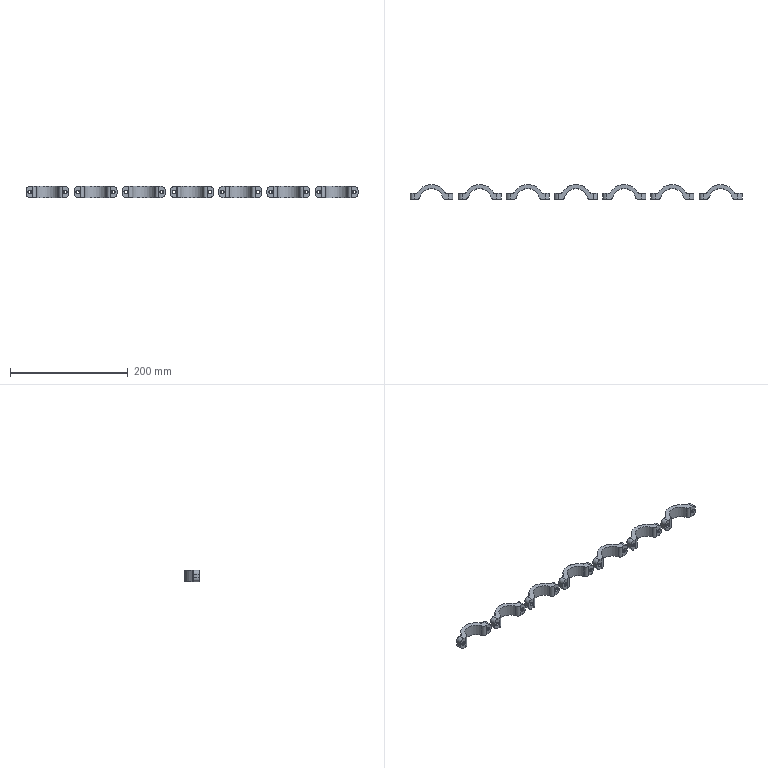NC program | Mastercam | posted with a generic post
Lines 2923 to 4896 of 23883, first 1623 of 1974 lines:
(16 CO |TOOL - 1|DIA. OFF. - 1|LEN. - 1|TOOL DIA. - 16.)
N5908 T1 M6
N5910 G0 G56 G90 X-44.884 Y-23.028 C0. B180. S6000 M3
N5912 G43 H1 Z40.
N5914 Z23.
N5916 G1 Z20.35 F2000.
N5918 X-45.357 Y-21.853 Z20.234 F4000.
N5920 G3 X-46.151 Y-20.651 Z20.1 I-3.34 J-1.343
N5922 G1 X-46.65 Y-19.858
N5924 G2 X-48.163 Y-14.465 I12.434 J6.398
N5926 X-48.3 Y-10.792 I49.344 J3.673
N5928 X-48.298 Y-10.346 I49.481
N5930 X-48.271 Y-4.938 I865.739 J-1.617
N5932 G1 X-48.266 Y-4.342
N5934 X-48.146 Y12.852
N5936 G2 X-47.9 Y14.539 I7.703 J-.262
N5938 X-46.414 Y17.572 I8.353 J-2.211
N5940 X-43.642 Y20.06 I7.961 J-6.083
N5942 X-39.47 Y21.708 I7.094 J-11.854
N5944 X-35.506 Y22.258 I5.523 J-25.257
N5946 X-30.242 Y22.416 I5.264 J-87.34
N5948 X-29.657 Y22.414 J-87.498
N5950 X-22.977 Y22.386 I-.5 J-912.012
N5952 G1 X-22.373 Y22.382
N5954 X33.907 Y22.008
N5956 X34.201 Y22.009
N5958 G2 X37.187 Y21.983 J-172.847
N5960 X40.482 Y20.969 I-.705 J-8.148
N5962 X43.577 Y18.308 I-5.14 J-9.11
N5964 X45.609 Y14.702 I-11.006 J-8.578
N5966 X46.723 Y10.602 I-19.798 J-7.578
N5968 X47.299 Y4.944 I-46.088 J-7.548
N5970 X47.479 Y-3.923 I-217.933 J-8.867
N5972 G1 Y-3.929
N5974 G2 X47.489 Y-6.4 I-975.272 J-5.162
N5976 G1 X47.49 Y-7.016
N5978 G2 X47.494 Y-9.105 I-595.573 J-2.089
N5980 X47.49 Y-11.453 I-595.577
N5982 X46.583 Y-14.751 I-8.028 J.432
N5984 X43.991 Y-17.922 I-9.082 J4.78
N5986 X39.944 Y-20.204 I-8.744 J10.774
N5988 X35.874 Y-21.26 I-7.5 J20.538
N5990 X30.245 Y-21.807 I-7.504 J47.966
N5992 X21.392 Y-21.979 I-8.853 J227.798
N5994 G1 X21.385
N5996 G2 X19.531 Y-21.987 I-4.737 J921.856
N5998 G1 X18.915 Y-21.989
N6000 X-36.463 Y-21.993
N6002 G2 X-40.392 Y-20.823 I.404 J8.545
N6004 X-43.439 Y-18.134 I5.427 J9.217
N6006 X-45.439 Y-14.523 I11.134 J8.529
N6008 X-46.528 Y-10.416 I19.842 J7.456
N6010 X-47.067 Y-4.751 I45.995 J7.238
N6012 X-47.192 Y2.627 I217.088 J7.378
N6014 X-47.187 Y4.123 I217.213
N6016 X-47.18 Y6.594 I970.906 J-1.502
N6018 G1 X-47.178 Y7.21
N6020 G2 X-47.155 Y9.304 I114.207 J-.216
N6022 X-44.591 Y15.696 I10.476 J-.491
N6024 X-40.819 Y18.674 I9.729 J-8.446
N6026 X-36.989 Y20.159 I8.291 J-15.701
N6028 X-32.412 Y20.97 I7.487 J-28.95
N6030 X-26.367 Y21.299 I6.984 J-72.475
N6032 X-19.406 Y21.346 I6.961 J-512.395
N6034 X-14.54 Y21.324 J-512.442
N6036 G1 X-13.926 Y21.32
N6038 X33.206 Y21.005
N6040 G2 X40.416 Y18.047 I-.442 J-11.343
N6042 X43.518 Y13.986 I-9.563 J-10.518
N6044 X45.177 Y9.517 I-18.069 J-9.253
N6046 X46.028 Y4.379 I-34.271 J-8.311
N6048 X46.404 Y-2.851 I-94.948 J-8.563
N6050 X46.464 Y-7.318 I-291.246 J-6.155
N6052 X43.757 Y-14.636 I-11.254 J.003
N6054 X39.738 Y-17.867 I-10.573 J9.037
N6056 X35.25 Y-19.611 I-9.342 J17.402
N6058 X30.082 Y-20.504 I-8.375 J33.036
N6060 X23.468 Y-20.883 I-8.361 J88.08
N6062 X12.151 Y-20.995 I-11.317 J576.455
N6064 X11.038 Y-20.993 J576.566
N6066 G1 X10.423 Y-20.994
N6068 X-32.667 Y-20.995
N6070 G2 X-40.331 Y-17.889 I.182 J11.455
N6072 X-43.371 Y-13.804 I9.797 J10.466
N6074 X-44.985 Y-9.33 I18.285 J9.126
N6076 X-45.795 Y-4.192 I34.546 J8.076
N6078 X-46.12 Y3.038 I95.438 J7.911
N6080 X-46.139 Y5.321 I135.435 J2.283
N6082 G1 Y5.679
N6084 G2 X-45.662 Y9.236 I13.643 J-.018
N6086 X-42.309 Y14.816 I11.969 J-3.393
N6088 X-38.661 Y17.41 I10.477 J-10.873
N6090 X-33.842 Y19.148 I9.553 J-18.94
N6092 X-28.045 Y20.004 I8.556 J-37.876
N6094 X-20.243 Y20.292 I8.196 J-116.201
N6096 X-14.949 Y20.306 I5.294 J-980.054
N6098 X-6.64 Y20.272 J-980.068
N6100 G1 X-6.026 Y20.267
N6102 X29.631 Y20.027
N6104 G2 X32.943 Y19.666 I-.08 J-16.055
N6106 X39.744 Y15.722 I-2.916 J-12.866
N6108 X42.235 Y12.172 I-11.816 J-10.939
N6110 X44.013 Y7.445 I-19.674 J-10.101
N6112 X44.986 Y1.662 I-37.574 J-9.294
N6114 X45.331 Y-4.52 I-76.625 J-7.38
N6116 G1 Y-4.572
N6118 G2 X44.35 Y-9.632 I-13.534
N6120 X40.614 Y-14.709 I-12.401 J5.213
N6122 X36.622 Y-17.211 I-10.844 J12.861
N6124 X31.942 Y-18.74 I-9.756 J21.949
N6126 X26.25 Y-19.565 I-9.037 J42.276
N6128 X18.472 Y-19.911 I-9.295 J121.207
N6130 X5.449 Y-19.998 I-13.023 J981.766
N6132 X3.633 Y-19.996 J981.852
N6134 G1 X3.019 Y-19.997
N6136 X-29.668 Y-19.988
N6138 G2 X-33.578 Y-19.409 I.23 J15.043
N6140 X-39.75 Y-15.436 I3.847 J12.756
N6142 X-42.342 Y-11.461 I12.349 J10.885
N6144 X-43.932 Y-6.754 I21.156 J9.768
N6146 X-44.776 Y-1.022 I40.362 J8.873
N6148 X-44.986 Y3.21 I56.386 J4.914
N6150 G1 Y3.27
N6152 G2 X-44.508 Y7.095 I15.548
N6154 X-40.431 Y13.721 I13.097 J-3.49
N6156 X-36.503 Y16.346 I11.107 J-12.37
N6158 X-31.807 Y17.997 I9.983 J-20.892
N6160 X-26.055 Y18.897 I9.071 J-39.163
N6162 X-18.221 Y19.248 I8.743 J-107.429
N6164 X-10.9 Y19.282 I7.321 J-771.653
N6166 X-3.975 Y19.252 J-771.688
N6168 G1 X-3.361 Y19.247
N6170 X26.781 Y19.041
N6172 G2 X30.135 Y18.763 I-.157 J-22.182
N6174 X38.782 Y13.854 I-2.371 J-14.247
N6176 X41.647 Y9.224 I-13.729 J-11.7
N6178 X43.283 Y3.902 I-24.295 J-10.377
N6180 X43.984 Y-1.194 I-40.547 J-8.179
N6182 X44.032 Y-2.454 I-16.613 J-1.26
N6184 X43.845 Y-4.947 I-16.661
N6186 X39.813 Y-12.677 I-13.559 J2.155
N6188 X35.994 Y-15.454 I-11.605 J11.941
N6190 X31.333 Y-17.29 I-10.585 J20.049
N6192 X25.548 Y-18.365 I-9.808 J36.689
N6194 X18.292 Y-18.838 I-9.436 J88.748
N6196 X6.377 Y-18.988 I-11.915 J476.068
N6198 G1 X5.836 Y-18.987
N6200 X5.221 Y-18.989
N6202 X-26.132 Y-18.996
N6204 X-26.274 Y-18.997
N6206 G2 X-29.815 Y-18.736 J24.22
N6208 X-38.503 Y-13.872 I2.246 J14.205
N6210 X-41.025 Y-10.018 I13.181 J11.376
N6212 X-42.862 Y-4.63 I22.04 J10.522
N6214 X-43.62 Y.675 I32.605 J7.367
N6216 X-43.646 Y1.583 I16.129 J.908
N6218 X-43.281 Y4.996 I16.155
N6220 X-39.255 Y12.078 I13.734 J-3.122
N6222 X-35.448 Y14.821 I11.701 J-12.225
N6224 X-30.793 Y16.651 I10.619 J-20.178
N6226 X-24.996 Y17.724 I9.721 J-36.329
N6228 X-17.721 Y18.175 I8.973 J-85.833
N6230 X-9.051 Y18.265 I8.67 J-416.715
N6232 X-5.867 Y18.253 J-416.805
N6234 G1 X-5.251 Y18.25
N6236 X24.308 Y18.053
N6238 G2 X28.281 Y17.719 I-.281 J-27.075
N6240 X37.8 Y12.131 I-2.537 J-15.223
N6242 X40.684 Y7.207 I-15.183 J-12.199
N6244 X42.373 Y.943 I-24.077 J-9.853
N6246 X42.521 Y-1.199 I-15.427 J-2.142
N6248 X42.36 Y-3.43 I-15.575
N6250 X38.48 Y-11.166 I-13.844 J2.102
N6252 X34.754 Y-14.034 I-12.038 J11.786
N6254 X30.132 Y-16.005 I-11.068 J19.551
N6256 X24.322 Y-17.219 I-10.291 J34.76
N6258 X17.011 Y-17.787 I-9.856 J79.506
N6260 X5.747 Y-17.975 I-11.505 J350.541
N6262 G1 X5.13 Y-17.979
N6264 X-23.151 Y-17.997
N6266 X-23.307 Y-17.998
N6268 G2 X-26.853 Y-17.834 J38.682
N6270 X-31.433 Y-16.701 I1.631 J16.421
N6272 X-37.658 Y-11.971 I5.985 J14.336
N6274 X-40.331 Y-7.413 I15.207 J11.981
N6276 X-41.916 Y-1.779 I21.451 J9.077
N6278 X-42.085 Y.483 I15.043 J2.262
N6280 X-41.854 Y3.127 I15.212
N6282 X-38.138 Y10.37 I13.894 J-2.553
N6284 X-34.443 Y13.281 I12.146 J-11.614
N6286 X-29.818 Y15.303 I11.138 J-19.183
N6288 X-23.981 Y16.547 I10.247 J-33.756
N6290 X-16.638 Y17.109 I9.482 J-75.712
N6292 X-7.264 Y17.244 I9.374 J-324.031
N6294 X-5.355 Y17.238 J-324.167
N6296 G1 X-4.737 Y17.237
N6298 X20.461 Y17.087
N6300 X20.546 Y17.088
N6302 G2 X24.644 Y16.932 J-54.062
N6304 X28.969 Y16.079 I-1.525 J-19.123
N6306 X36.14 Y11.319 I-5.025 J-15.352
N6308 X39.713 Y5.273 I-14.857 J-12.86
N6310 X40.707 Y1.143 I-15.557 J-5.927
N6312 X40.786 Y-.32 I-13.573 J-1.463
N6314 X37.607 Y-9.076 I-13.652
N6316 X34.032 Y-12.278 I-12.441 J10.295
N6318 X29.438 Y-14.551 I-11.6 J17.67
N6320 X23.563 Y-16.004 I-10.813 J31.123
N6322 X16.813 Y-16.679 I-10.074 J66.612
N6324 X6.702 Y-16.949 I-11.173 J228.959
N6326 X-.09 Y-16.986 I-8.808 J997.7
N6328 G1 X-.706 Y-16.988
N6330 X-21.016 Y-16.994
N6332 G2 X-24.622 Y-16.844 I.04 J44.664
N6334 X-29.005 Y-15.932 I1.558 J18.48
N6336 X-35.794 Y-11.389 I5.229 J15.156
N6338 X-39.84 Y-3.807 I13.83 J12.252
N6340 X-40.286 Y-.322 I13.407 J3.485
N6342 X-39.777 Y3.396 I13.853
N6344 X-36.113 Y9.533 I13.638 J-3.981
N6346 X-32.018 Y12.544 I12.215 J-12.321
N6348 X-26.682 Y14.601 I11.262 J-21.27
N6350 X-20.282 Y15.705 I10.275 J-40.457
N6352 X-12.433 Y16.143 I9.662 J-102.647
N6354 X-3.307 Y16.225 I9.126 J-507.263
N6356 X.629 Y16.21 J-507.345
N6358 G1 X1.245 Y16.207
N6360 X19.105 Y16.09
N6362 G2 X23.376 Y15.87 I-.217 J-45.652
N6364 X28.067 Y14.801 I-1.99 J-19.558
N6366 X36.683 Y7.65 I-5.93 J-15.91
N6368 X38.641 Y2.437 I-12.424 J-7.643
N6370 X38.804 Y.393 I-12.752 J-2.044
N6372 X36.615 Y-6.801 I-12.915
N6374 X32.866 Y-10.713 I-13.001 J8.707
N6376 X28.293 Y-13.215 I-11.853 J16.237
N6378 X23.092 Y-14.706 I-10.725 J27.591
N6380 X16.232 Y-15.569 I-10.502 J55.778
N6382 X7.293 Y-15.909 I-10.803 J166.404
N6384 X-5.24 Y-15.992 I-12.533 J949.534
N6386 X-5.685 Y-15.991 J949.617
N6388 G1 X-6.3 Y-15.993
N6390 X-19.273 Y-15.986
N6392 G2 X-23.662 Y-15.731 I.05 J38.732
N6394 X-28.427 Y-14.504 I2.225 J18.517
N6396 X-36.816 Y-6.792 I6.235 J15.199
N6398 X-38.235 Y-.894 I11.551 J5.898
N6400 X-38.205 Y-.032 I12.97
N6402 X-35.873 Y6.469 I12.933 J-.971
N6404 X-31.683 Y10.536 I12.669 J-8.861
N6406 X-27.085 Y12.828 I11.61 J-17.534
N6408 X-21.203 Y14.292 I10.813 J-30.899
N6410 X-14.437 Y14.965 I9.881 J-64.995
N6412 X-4.472 Y15.197 I9.965 J-213.659
N6414 G1 X-4.304
N6416 G2 X-1.177 Y15.202 I3.127 J-959.648
N6418 X3.726 Y15.189 J-959.653
N6420 G1 X4.342 Y15.186
N6422 X17.31 Y15.096
N6424 G2 X21.539 Y14.876 I-.44 J-48.99
N6426 X26.532 Y13.772 I-2.04 J-21.08
N6428 X32.909 Y9.668 I-5.584 J-15.683
N6430 X35.954 Y4.72 I-9.601 J-9.319
N6432 X36.567 Y.947 I-11.302 J-3.773
N6434 X35.493 Y-3.998 I-11.915
N6436 X31.799 Y-8.9 I-13.003 J5.955
N6438 X27.621 Y-11.598 I-11.773 J13.646
N6440 X22.343 Y-13.406 I-11.099 J23.794
N6442 X16.048 Y-14.398 I-10.441 J45.811
N6444 X7.631 Y-14.852 I-10.685 J119.676
N6446 X-6.332 Y-14.99 I-13.963 J708.147
N6448 X-7.245 Y-14.989 J708.285
N6450 G1 X-7.859 Y-14.991
N6452 G2 X-11.297 Y-14.997 I-3.438 J898.451
N6454 X-17.808 Y-14.973 J898.458
N6456 X-22.206 Y-14.679 I.336 J38.047
N6458 X-27.313 Y-13.295 I2.468 J19.22
N6460 X-32.535 Y-9.681 I6.197 J14.535
N6462 X-35.506 Y-4.471 I8.96 J8.561
N6464 X-35.909 Y-1.431 I11.273 J3.04
N6466 X-34.928 Y3.252 I11.676
N6468 X-31.62 Y7.897 I12.723 J-5.563
N6470 X-27.836 Y10.559 I11.701 J-12.605
N6472 X-22.503 Y12.57 I11.191 J-21.605
N6474 X-16.129 Y13.653 I10.357 J-41.682
N6476 X-8.292 Y14.097 I9.87 J-104.79
N6478 X1.247 Y14.19 I9.539 J-487.809
N6480 X4.776 Y14.177 J-487.902
N6482 G1 X5.392 Y14.175
N6484 X15.295 Y14.107
N6486 G2 X20.201 Y13.836 I-.461 J-52.82
N6488 X25.141 Y12.714 I-2.345 J-21.763
N6490 X29.399 Y10.429 I-5.404 J-15.179
N6492 X32.681 Y6.689 I-7.346 J-9.755
N6494 X34.027 Y1.433 I-9.587 J-5.256
N6496 X33.71 Y-1.177 I-10.933
N6498 X30.967 Y-6.439 I-12.307 J3.07
N6500 X27.264 Y-9.575 I-11.897 J10.295
N6502 X22.644 Y-11.699 I-11.3 J18.495
N6504 X16.823 Y-13.033 I-10.744 J33.49
N6506 X9.478 Y-13.702 I-10.466 J74.315
N6508 X-1.211 Y-13.952 I-11.702 J271.761
N6510 X-5.534 Y-13.977 I-7.889 J968.44
N6512 G1 X-6.15 Y-13.98
N6514 G2 X-10.115 Y-13.993 I-3.965 J647.904
N6516 X-16.127 Y-13.964 J647.916
N6518 X-20.481 Y-13.674 I.508 J40.507
N6520 X-25.085 Y-12.561 I2.503 J20.423
N6522 X-29.05 Y-10.367 I5.164 J14.011
N6524 X-32.502 Y-5.828 I6.779 J8.738
N6526 X-33.253 Y-1.88 I10.007 J3.948
N6528 X-32.848 Y1.044 I10.758
N6530 X-29.926 Y6.207 I12.193 J-3.491
N6532 X-26.541 Y8.972 I11.59 J-10.732
N6534 X-21.897 Y11.078 I11.131 J-18.371
N6536 X-16.063 Y12.374 I10.49 J-33.447
N6538 X-8.714 Y12.991 I9.952 J-74.522
N6540 X1.47 Y13.17 I10.184 J-289.084
N6542 X2.595 Y13.168 J-289.263
N6544 G1 X3.181
N6546 G2 X5.683 Y13.165 J-974.104
N6548 G1 X6.299 Y13.163
N6550 G2 X14.421 Y13.093 I-.2 J-495.657
N6552 X19.441 Y12.724 I-.758 J-44.556
N6554 X24.05 Y11.546 I-2.741 J-20.34
N6556 X27.769 Y9.321 I-4.444 J-11.647
N6558 X31.128 Y1.893 I-6.534 J-7.428
N6560 X31.065 Y.782 I-9.893
N6562 X29.087 Y-4.48 I-11.427 J1.293
N6564 X25.098 Y-8.36 I-11.91 J8.252
N6566 X20.429 Y-10.631 I-11.181 J17.052
N6568 X14.562 Y-12.02 I-10.652 J31.926
N6570 X7.201 Y-12.699 I-10.409 J72.593
N6572 X-3.49 Y-12.95 I-11.721 J270.501
N6574 X-8.431 Y-12.979 I-8.146 J995.561
N6576 X-10.273 Y-12.987 I-1.842 J217.156
N6578 X-15.437 Y-12.925 J217.164
N6580 X-19.911 Y-12.508 I.967 J34.557
N6582 X-23.388 Y-11.595 I3.045 J18.675
N6584 X-26.785 Y-9.655 I4.018 J10.981
N6586 X-30.2 Y-2.348 I6.11 J7.307
N6588 X-30.179 Y-1.707 I9.525
N6590 X-28.651 Y3.21 I10.99 J-.718
N6592 X-25.167 Y7.101 I11.871 J-7.125
N6594 X-20.83 Y9.54 I10.916 J-14.334
N6596 X-15.553 Y11.043 I10.265 J-26.021
N6598 X-9.344 Y11.807 I9.647 J-52.804
N6600 X-.376 Y12.122 I9.935 J-154.892
N6602 X5.109 Y12.151 I5.485 J-507.313
N6604 X12.749 Y12.094 J-507.343
N6606 X17.724 Y11.744 I-.845 J-47.461
N6608 X21.171 Y10.989 I-2.554 J-19.925
N6610 X24.261 Y9.402 I-3.121 J-9.877
N6612 X27.69 Y3.33 I-5.382 J-7.043
N6614 X27.751 Y2.225 I-10.015 J-1.105
N6616 X26.881 Y-1.871 I-10.076
N6618 X23.658 Y-6.234 I-11.547 J5.157
N6620 X20.482 Y-8.416 I-10.607 J12.04
N6622 X15.806 Y-10.22 I-10.458 J20.141
N6624 X10.066 Y-11.276 I-10.048 J38.489
N6626 X2.194 Y-11.802 I-10.464 J97.405
N6628 X-8.792 Y-11.961 I-10.986 J380.97
N6630 X-12.892 Y-11.938 J381.128
N6632 X-17.181 Y-11.663 I.699 J44.352
N6634 X-20.313 Y-11.033 I2.009 J18.109
N6636 X-23.444 Y-9.401 I2.658 J8.919
N6638 X-26.524 Y-3.846 I5.38 J6.613
N6640 X-26.601 Y-2.626 I9.663 J1.22
N6642 X-25.964 Y.839 I9.74
N6644 X-23.234 Y5.036 I11.108 J-4.237
N6646 X-19.251 Y7.897 I10.824 J-10.866
N6648 X-14.551 Y9.63 I10.162 J-20.324
N6650 X-8.814 Y10.606 I9.626 J-39.224
N6652 X-.957 Y11.051 I9.674 J-101.283
N6654 X5.912 Y11.129 I6.869 J-300.508
N6656 X11.667 Y11.074 J-300.586
N6658 X15.977 Y10.764 I-1.019 J-44.25
N6660 X17.981 Y10.363 I-1.681 J-13.615
N6662 X23.406 Y4.909 I-2.127 J-7.542
N6664 X23.734 Y2.494 I-8.716 J-2.415
N6666 X23.437 Y.193 I-9.044
N6668 X21.003 Y-4.332 I-10.676 J2.826
N6670 X17.017 Y-7.468 I-10.778 J9.596
N6672 X12.263 Y-9.323 I-10.131 J18.951
N6674 X6.496 Y-10.347 I-9.69 J37.822
N6676 X-1.357 Y-10.828 I-10.18 J101.794
N6678 X-8.344 Y-10.934 I-6.987 J230.985
N6680 X-11.519 Y-10.912 J231.091
N6682 X-15.621 Y-10.633 I.545 J38.365
N6684 X-18.767 Y-9.503 I.995 J7.712
N6686 X-21.752 Y-5.687 I4.02 J6.221
N6688 X-22.216 Y-2.894 I8.179 J2.793
N6690 X-22.121 Y-1.613 I8.643
N6692 X-20.37 Y2.726 I10.081 J-1.544
N6694 X-16.915 Y6.073 I10.543 J-7.43
N6696 X-12.808 Y8.088 I9.767 J-14.71
N6698 X-7.517 Y9.344 I9.316 J-27.474
N6700 X-.743 Y9.94 I9.195 J-65.666
N6702 X6.41 Y10.089 I7.153 J-171.222
N6704 X10.826 Y10.033 J-171.371
N6706 X12.753 Y9.913 I-1.151 J-34.045
N6708 X13.754 Y9.713 I-.842 J-6.828
N6710 G1 X14.603 Y9.411
N6712 X15.39 Y9.
N6714 X16.119 Y8.477
N6716 G2 X18.322 Y5.039 I-4.431 J-5.264
N6718 X18.625 Y2.776 I-8.29 J-2.263
N6720 X18.438 Y.991 I-8.593
N6722 X16.434 Y-3.24 I-10.097 J2.192
N6724 X12.821 Y-6.372 I-10.176 J8.088
N6726 X9.101 Y-8.046 I-9.239 J15.564
N6728 X3.832 Y-9.213 I-9.092 J28.559
N6730 X-2.891 Y-9.763 I-9.224 J71.369
N6732 X-8.012 Y-9.878 I-5.121 J114.655
N6734 X-10.77 Y-9.845 J114.769
N6736 G1 X-11.566 Y-9.738
N6738 X-12.295 Y-9.537
N6740 X-12.985 Y-9.243
N6742 X-13.644 Y-8.848
N6744 X-14.269 Y-8.344
N6746 X-14.843 Y-7.722
N6748 X-15.35 Y-6.986
N6750 G2 X-16.272 Y-3.969 I6.141 J3.526
N6752 X-16.295 Y-3.333 I8.713 J.636
N6754 X-15.821 Y-.496 I8.736
N6756 X-13.004 Y3.895 I10.488 J-3.63
N6758 X-9.179 Y6.493 I9.679 J-10.136
N6760 X-5.114 Y7.887 I8.659 J-18.622
N6762 X-.007 Y8.687 I8.217 J-35.776
N6764 X6.605 Y8.997 I7.077 J-80.228
N6766 X9.31 Y8.169 I-.233 J-5.595
N6768 G1 X9.945 Y7.713
N6770 X10.589 Y7.085
N6772 G2 X11.721 Y5.132 I-4.66 J-4.002
N6774 X12.174 Y2.494 I-7.455 J-2.638
N6776 X12.145 Y1.817 I-7.908
N6778 X11.127 Y-1.627 I-8.967 J.776
N6780 X8.175 Y-5.172 I-9.983 J5.312
N6782 X4.425 Y-7.28 I-8.554 J10.827
N6784 X.345 Y-8.366 I-7.583 J20.295
N6786 X-3.662 Y-8.825 I-6.319 J37.465
N6788 X-3.794 Y-8.827 I-.132 J5.599
N6790 X-5.835 Y-8.441 J5.601
N6792 G1 X-6.596 Y-8.075
N6794 G2 X-8.035 Y-6.883 I2.904 J4.972
N6796 X-8.879 Y-5.612 I4.798 J4.098
N6798 G1 X-9.211 Y-4.847
N6800 X-9.468 Y-3.997
N6802 X-9.631 Y-3.083
N6804 X-9.686 Y-2.119
N6806 X-9.625 Y-1.132
N6808 X-9.449 Y-.146
N6810 X-9.161 Y.813
N6812 X-8.776 Y1.724
N6814 G2 X-7.2 Y4.036 I8.815 J-4.317
N6816 X-3.546 Y6.713 I8.652 J-7.976
N6818 X-1.693 Y7.421 I4.944 J-10.154
N6820 G1 X1.801 Y8.289 Z20.35
N6822 G0 Z40.
N6824 X-44.884 Y-23.028
N6826 Z23.
N6828 G1 Z20.35 F2000.
N6830 X-45.357 Y-21.853 Z20.234 F4000.
N6832 G3 X-46.151 Y-20.651 Z20.1 I-3.34 J-1.343
N6834 G1 X-46.65 Y-19.858
N6836 G2 X-48.163 Y-14.465 I12.434 J6.398
N6838 X-48.3 Y-10.792 I49.344 J3.673
N6840 X-48.298 Y-10.346 I49.481
N6842 X-48.271 Y-4.938 I865.739 J-1.617
N6844 G1 X-48.266 Y-4.342
N6846 X-48.146 Y12.852
N6848 G2 X-47.9 Y14.539 I7.703 J-.262
N6850 X-46.414 Y17.572 I8.353 J-2.211
N6852 X-43.642 Y20.06 I7.961 J-6.083
N6854 X-39.47 Y21.708 I7.094 J-11.854
N6856 X-35.506 Y22.258 I5.523 J-25.257
N6858 X-30.242 Y22.416 I5.264 J-87.34
N6860 X-29.657 Y22.414 J-87.498
N6862 X-22.977 Y22.386 I-.5 J-912.012
N6864 G1 X-22.373 Y22.382
N6866 X33.907 Y22.008
N6868 X34.201 Y22.009
N6870 G2 X37.187 Y21.983 J-172.847
N6872 X40.482 Y20.969 I-.705 J-8.148
N6874 X43.577 Y18.308 I-5.14 J-9.11
N6876 X45.609 Y14.702 I-11.006 J-8.578
N6878 X46.723 Y10.602 I-19.798 J-7.578
N6880 X47.299 Y4.944 I-46.088 J-7.548
N6882 X47.479 Y-3.923 I-217.933 J-8.867
N6884 G1 Y-3.929
N6886 G2 X47.489 Y-6.4 I-975.272 J-5.162
N6888 G1 X47.49 Y-7.016
N6890 G2 X47.494 Y-9.105 I-595.573 J-2.089
N6892 X47.49 Y-11.453 I-595.577
N6894 X46.583 Y-14.751 I-8.028 J.432
N6896 X43.991 Y-17.922 I-9.082 J4.78
N6898 X39.944 Y-20.204 I-8.744 J10.774
N6900 X35.874 Y-21.26 I-7.5 J20.538
N6902 X30.245 Y-21.807 I-7.504 J47.966
N6904 X21.392 Y-21.979 I-8.853 J227.798
N6906 G1 X21.385
N6908 G2 X19.531 Y-21.987 I-4.737 J921.856
N6910 G1 X18.915 Y-21.989
N6912 X-36.463 Y-21.993
N6914 G2 X-40.392 Y-20.823 I.404 J8.545
N6916 X-43.439 Y-18.134 I5.427 J9.217
N6918 X-45.439 Y-14.523 I11.134 J8.529
N6920 X-46.528 Y-10.416 I19.842 J7.456
N6922 X-47.067 Y-4.751 I45.995 J7.238
N6924 X-47.192 Y2.627 I217.088 J7.378
N6926 X-47.187 Y4.123 I217.213
N6928 X-47.18 Y6.594 I970.906 J-1.502
N6930 G1 X-47.178 Y7.21
N6932 G2 X-47.155 Y9.304 I114.207 J-.216
N6934 X-44.591 Y15.696 I10.476 J-.491
N6936 X-40.819 Y18.674 I9.729 J-8.446
N6938 X-36.989 Y20.159 I8.291 J-15.701
N6940 X-32.412 Y20.97 I7.487 J-28.95
N6942 X-26.367 Y21.299 I6.984 J-72.475
N6944 X-19.406 Y21.346 I6.961 J-512.395
N6946 X-14.54 Y21.324 J-512.442
N6948 G1 X-13.926 Y21.32
N6950 X33.206 Y21.005
N6952 G2 X40.416 Y18.047 I-.442 J-11.343
N6954 X43.518 Y13.986 I-9.563 J-10.518
N6956 X45.177 Y9.517 I-18.069 J-9.253
N6958 X46.028 Y4.379 I-34.271 J-8.311
N6960 X46.404 Y-2.851 I-94.948 J-8.563
N6962 X46.464 Y-7.318 I-291.246 J-6.155
N6964 X43.757 Y-14.636 I-11.254 J.003
N6966 X39.738 Y-17.867 I-10.573 J9.037
N6968 X35.25 Y-19.611 I-9.342 J17.402
N6970 X30.082 Y-20.504 I-8.375 J33.036
N6972 X23.468 Y-20.883 I-8.361 J88.08
N6974 X12.151 Y-20.995 I-11.317 J576.455
N6976 X11.038 Y-20.993 J576.566
N6978 G1 X10.423 Y-20.994
N6980 X-32.667 Y-20.995
N6982 G2 X-40.331 Y-17.889 I.182 J11.455
N6984 X-43.371 Y-13.804 I9.797 J10.466
N6986 X-44.985 Y-9.33 I18.285 J9.126
N6988 X-45.795 Y-4.192 I34.546 J8.076
N6990 X-46.12 Y3.038 I95.438 J7.911
N6992 X-46.139 Y5.321 I135.435 J2.283
N6994 G1 Y5.679
N6996 G2 X-45.662 Y9.236 I13.643 J-.018
N6998 X-42.309 Y14.816 I11.969 J-3.393
N7000 X-38.661 Y17.41 I10.477 J-10.873
N7002 X-33.842 Y19.148 I9.553 J-18.94
N7004 X-28.045 Y20.004 I8.556 J-37.876
N7006 X-20.243 Y20.292 I8.196 J-116.201
N7008 X-14.949 Y20.306 I5.294 J-980.054
N7010 X-6.64 Y20.272 J-980.068
N7012 G1 X-6.026 Y20.267
N7014 X29.631 Y20.027
N7016 G2 X32.943 Y19.666 I-.08 J-16.055
N7018 X39.744 Y15.722 I-2.916 J-12.866
N7020 X42.235 Y12.172 I-11.816 J-10.939
N7022 X44.013 Y7.445 I-19.674 J-10.101
N7024 X44.986 Y1.662 I-37.574 J-9.294
N7026 X45.331 Y-4.52 I-76.625 J-7.38
N7028 G1 Y-4.572
N7030 G2 X44.35 Y-9.632 I-13.534
N7032 X40.614 Y-14.709 I-12.401 J5.213
N7034 X36.622 Y-17.211 I-10.844 J12.861
N7036 X31.942 Y-18.74 I-9.756 J21.949
N7038 X26.25 Y-19.565 I-9.037 J42.276
N7040 X18.472 Y-19.911 I-9.295 J121.207
N7042 X5.449 Y-19.998 I-13.023 J981.766
N7044 X3.633 Y-19.996 J981.852
N7046 G1 X3.019 Y-19.997
N7048 X-29.668 Y-19.988
N7050 G2 X-33.578 Y-19.409 I.23 J15.043
N7052 X-39.75 Y-15.436 I3.847 J12.756
N7054 X-42.342 Y-11.461 I12.349 J10.885
N7056 X-43.932 Y-6.754 I21.156 J9.768
N7058 X-44.776 Y-1.022 I40.362 J8.873
N7060 X-44.986 Y3.21 I56.386 J4.914
N7062 G1 Y3.27
N7064 G2 X-44.508 Y7.095 I15.548
N7066 X-40.431 Y13.721 I13.097 J-3.49
N7068 X-36.503 Y16.346 I11.107 J-12.37
N7070 X-31.807 Y17.997 I9.983 J-20.892
N7072 X-26.055 Y18.897 I9.071 J-39.163
N7074 X-18.221 Y19.248 I8.743 J-107.429
N7076 X-10.9 Y19.282 I7.321 J-771.653
N7078 X-3.975 Y19.252 J-771.688
N7080 G1 X-3.361 Y19.247
N7082 X26.781 Y19.041
N7084 G2 X30.135 Y18.763 I-.157 J-22.182
N7086 X38.782 Y13.854 I-2.371 J-14.247
N7088 X41.647 Y9.224 I-13.729 J-11.7
N7090 X43.283 Y3.902 I-24.295 J-10.377
N7092 X43.984 Y-1.194 I-40.547 J-8.179
N7094 X44.032 Y-2.454 I-16.613 J-1.26
N7096 X43.845 Y-4.947 I-16.661
N7098 X39.813 Y-12.677 I-13.559 J2.155
N7100 X35.994 Y-15.454 I-11.605 J11.941
N7102 X31.333 Y-17.29 I-10.585 J20.049
N7104 X25.548 Y-18.365 I-9.808 J36.689
N7106 X18.292 Y-18.838 I-9.436 J88.748
N7108 X6.377 Y-18.988 I-11.915 J476.068
N7110 G1 X5.836 Y-18.987
N7112 X5.221 Y-18.989
N7114 X-26.132 Y-18.996
N7116 X-26.274 Y-18.997
N7118 G2 X-29.815 Y-18.736 J24.22
N7120 X-38.503 Y-13.872 I2.246 J14.205
N7122 X-41.025 Y-10.018 I13.181 J11.376
N7124 X-42.862 Y-4.63 I22.04 J10.522
N7126 X-43.62 Y.675 I32.605 J7.367
N7128 X-43.646 Y1.583 I16.129 J.908
N7130 X-43.281 Y4.996 I16.155
N7132 X-39.255 Y12.078 I13.734 J-3.122
N7134 X-35.448 Y14.821 I11.701 J-12.225
N7136 X-30.793 Y16.651 I10.619 J-20.178
N7138 X-24.996 Y17.724 I9.721 J-36.329
N7140 X-17.721 Y18.175 I8.973 J-85.833
N7142 X-9.051 Y18.265 I8.67 J-416.715
N7144 X-5.867 Y18.253 J-416.805
N7146 G1 X-5.251 Y18.25
N7148 X24.308 Y18.053
N7150 G2 X28.281 Y17.719 I-.281 J-27.075
N7152 X37.8 Y12.131 I-2.537 J-15.223
N7154 X40.684 Y7.207 I-15.183 J-12.199
N7156 X42.373 Y.943 I-24.077 J-9.853
N7158 X42.521 Y-1.199 I-15.427 J-2.142
N7160 X42.36 Y-3.43 I-15.575
N7162 X38.48 Y-11.166 I-13.844 J2.102
N7164 X34.754 Y-14.034 I-12.038 J11.786
N7166 X30.132 Y-16.005 I-11.068 J19.551
N7168 X24.322 Y-17.219 I-10.291 J34.76
N7170 X17.011 Y-17.787 I-9.856 J79.506
N7172 X5.747 Y-17.975 I-11.505 J350.541
N7174 G1 X5.13 Y-17.979
N7176 X-23.151 Y-17.997
N7178 X-23.307 Y-17.998
N7180 G2 X-26.853 Y-17.834 J38.682
N7182 X-31.433 Y-16.701 I1.631 J16.421
N7184 X-37.658 Y-11.971 I5.985 J14.336
N7186 X-40.331 Y-7.413 I15.207 J11.981
N7188 X-41.916 Y-1.779 I21.451 J9.077
N7190 X-42.085 Y.483 I15.043 J2.262
N7192 X-41.854 Y3.127 I15.212
N7194 X-38.138 Y10.37 I13.894 J-2.553
N7196 X-34.443 Y13.281 I12.146 J-11.614
N7198 X-29.818 Y15.303 I11.138 J-19.183
N7200 X-23.981 Y16.547 I10.247 J-33.756
N7202 X-16.638 Y17.109 I9.482 J-75.712
N7204 X-7.264 Y17.244 I9.374 J-324.031
N7206 X-5.355 Y17.238 J-324.167
N7208 G1 X-4.737 Y17.237
N7210 X20.461 Y17.087
N7212 X20.546 Y17.088
N7214 G2 X24.644 Y16.932 J-54.062
N7216 X28.969 Y16.079 I-1.525 J-19.123
N7218 X36.14 Y11.319 I-5.025 J-15.352
N7220 X39.713 Y5.273 I-14.857 J-12.86
N7222 X40.707 Y1.143 I-15.557 J-5.927
N7224 X40.786 Y-.32 I-13.573 J-1.463
N7226 X37.607 Y-9.076 I-13.652
N7228 X34.032 Y-12.278 I-12.441 J10.295
N7230 X29.438 Y-14.551 I-11.6 J17.67
N7232 X23.563 Y-16.004 I-10.813 J31.123
N7234 X16.813 Y-16.679 I-10.074 J66.612
N7236 X6.702 Y-16.949 I-11.173 J228.959
N7238 X-.09 Y-16.986 I-8.808 J997.7
N7240 G1 X-.706 Y-16.988
N7242 X-21.016 Y-16.994
N7244 G2 X-24.622 Y-16.844 I.04 J44.664
N7246 X-29.005 Y-15.932 I1.558 J18.48
N7248 X-35.794 Y-11.389 I5.229 J15.156
N7250 X-39.84 Y-3.807 I13.83 J12.252
N7252 X-40.286 Y-.322 I13.407 J3.485
N7254 X-39.777 Y3.396 I13.853
N7256 X-36.113 Y9.533 I13.638 J-3.981
N7258 X-32.018 Y12.544 I12.215 J-12.321
N7260 X-26.682 Y14.601 I11.262 J-21.27
N7262 X-20.282 Y15.705 I10.275 J-40.457
N7264 X-12.433 Y16.143 I9.662 J-102.647
N7266 X-3.307 Y16.225 I9.126 J-507.263
N7268 X.629 Y16.21 J-507.345
N7270 G1 X1.245 Y16.207
N7272 X19.105 Y16.09
N7274 G2 X23.376 Y15.87 I-.217 J-45.652
N7276 X28.067 Y14.801 I-1.99 J-19.558
N7278 X36.683 Y7.65 I-5.93 J-15.91
N7280 X38.641 Y2.437 I-12.424 J-7.643
N7282 X38.804 Y.393 I-12.752 J-2.044
N7284 X36.615 Y-6.801 I-12.915
N7286 X32.866 Y-10.713 I-13.001 J8.707
N7288 X28.293 Y-13.215 I-11.853 J16.237
N7290 X23.092 Y-14.706 I-10.725 J27.591
N7292 X16.232 Y-15.569 I-10.502 J55.778
N7294 X7.293 Y-15.909 I-10.803 J166.404
N7296 X-5.24 Y-15.992 I-12.533 J949.534
N7298 X-5.685 Y-15.991 J949.617
N7300 G1 X-6.3 Y-15.993
N7302 X-19.273 Y-15.986
N7304 G2 X-23.662 Y-15.731 I.05 J38.732
N7306 X-28.427 Y-14.504 I2.225 J18.517
N7308 X-36.816 Y-6.792 I6.235 J15.199
N7310 X-38.235 Y-.894 I11.551 J5.898
N7312 X-38.205 Y-.032 I12.97
N7314 X-35.873 Y6.469 I12.933 J-.971
N7316 X-31.683 Y10.536 I12.669 J-8.861
N7318 X-27.085 Y12.828 I11.61 J-17.534
N7320 X-21.203 Y14.292 I10.813 J-30.899
N7322 X-14.437 Y14.965 I9.881 J-64.995
N7324 X-4.472 Y15.197 I9.965 J-213.659
N7326 G1 X-4.304
N7328 G2 X-1.177 Y15.202 I3.127 J-959.648
N7330 X3.726 Y15.189 J-959.653
N7332 G1 X4.342 Y15.186
N7334 X17.31 Y15.096
N7336 G2 X21.539 Y14.876 I-.44 J-48.99
N7338 X26.532 Y13.772 I-2.04 J-21.08
N7340 X32.909 Y9.668 I-5.584 J-15.683
N7342 X35.954 Y4.72 I-9.601 J-9.319
N7344 X36.567 Y.947 I-11.302 J-3.773
N7346 X35.493 Y-3.998 I-11.915
N7348 X31.799 Y-8.9 I-13.003 J5.955
N7350 X27.621 Y-11.598 I-11.773 J13.646
N7352 X22.343 Y-13.406 I-11.099 J23.794
N7354 X16.048 Y-14.398 I-10.441 J45.811
N7356 X7.631 Y-14.852 I-10.685 J119.676
N7358 X-6.332 Y-14.99 I-13.963 J708.147
N7360 X-7.245 Y-14.989 J708.285
N7362 G1 X-7.859 Y-14.991
N7364 G2 X-11.297 Y-14.997 I-3.438 J898.451
N7366 X-17.808 Y-14.973 J898.458
N7368 X-22.206 Y-14.679 I.336 J38.047
N7370 X-27.313 Y-13.295 I2.468 J19.22
N7372 X-32.535 Y-9.681 I6.197 J14.535
N7374 X-35.506 Y-4.471 I8.96 J8.561
N7376 X-35.909 Y-1.431 I11.273 J3.04
N7378 X-34.928 Y3.252 I11.676
N7380 X-31.62 Y7.897 I12.723 J-5.563
N7382 X-27.836 Y10.559 I11.701 J-12.605
N7384 X-22.503 Y12.57 I11.191 J-21.605
N7386 X-16.129 Y13.653 I10.357 J-41.682
N7388 X-8.292 Y14.097 I9.87 J-104.79
N7390 X1.247 Y14.19 I9.539 J-487.809
N7392 X4.776 Y14.177 J-487.902
N7394 G1 X5.392 Y14.175
N7396 X15.295 Y14.107
N7398 G2 X20.201 Y13.836 I-.461 J-52.82
N7400 X25.141 Y12.714 I-2.345 J-21.763
N7402 X29.399 Y10.429 I-5.404 J-15.179
N7404 X32.681 Y6.689 I-7.346 J-9.755
N7406 X34.027 Y1.433 I-9.587 J-5.256
N7408 X33.71 Y-1.177 I-10.933
N7410 X30.967 Y-6.439 I-12.307 J3.07
N7412 X27.264 Y-9.575 I-11.897 J10.295
N7414 X22.644 Y-11.699 I-11.3 J18.495
N7416 X16.823 Y-13.033 I-10.744 J33.49
N7418 X9.478 Y-13.702 I-10.466 J74.315
N7420 X-1.211 Y-13.952 I-11.702 J271.761
N7422 X-5.534 Y-13.977 I-7.889 J968.44
N7424 G1 X-6.15 Y-13.98
N7426 G2 X-10.115 Y-13.993 I-3.965 J647.904
N7428 X-16.127 Y-13.964 J647.916
N7430 X-20.481 Y-13.674 I.508 J40.507
N7432 X-25.085 Y-12.561 I2.503 J20.423
N7434 X-29.05 Y-10.367 I5.164 J14.011
N7436 X-32.502 Y-5.828 I6.779 J8.738
N7438 X-33.253 Y-1.88 I10.007 J3.948
N7440 X-32.848 Y1.044 I10.758
N7442 X-29.926 Y6.207 I12.193 J-3.491
N7444 X-26.541 Y8.972 I11.59 J-10.732
N7446 X-21.897 Y11.078 I11.131 J-18.371
N7448 X-16.063 Y12.374 I10.49 J-33.447
N7450 X-8.714 Y12.991 I9.952 J-74.522
N7452 X1.47 Y13.17 I10.184 J-289.084
N7454 X2.595 Y13.168 J-289.263
N7456 G1 X3.181
N7458 G2 X5.683 Y13.165 J-974.104
N7460 G1 X6.299 Y13.163
N7462 G2 X14.421 Y13.093 I-.2 J-495.657
N7464 X19.441 Y12.724 I-.758 J-44.556
N7466 X24.05 Y11.546 I-2.741 J-20.34
N7468 X27.769 Y9.321 I-4.444 J-11.647
N7470 X31.128 Y1.893 I-6.534 J-7.428
N7472 X31.065 Y.782 I-9.893
N7474 X29.087 Y-4.48 I-11.427 J1.293
N7476 X25.098 Y-8.36 I-11.91 J8.252
N7478 X20.429 Y-10.631 I-11.181 J17.052
N7480 X14.562 Y-12.02 I-10.652 J31.926
N7482 X7.201 Y-12.699 I-10.409 J72.593
N7484 X-3.49 Y-12.95 I-11.721 J270.501
N7486 X-8.431 Y-12.979 I-8.146 J995.561
N7488 X-10.273 Y-12.987 I-1.842 J217.156
N7490 X-15.437 Y-12.925 J217.164
N7492 X-19.911 Y-12.508 I.967 J34.557
N7494 X-23.388 Y-11.595 I3.045 J18.675
N7496 X-26.785 Y-9.655 I4.018 J10.981
N7498 X-30.2 Y-2.348 I6.11 J7.307
N7500 X-30.179 Y-1.707 I9.525
N7502 X-28.651 Y3.21 I10.99 J-.718
N7504 X-25.167 Y7.101 I11.871 J-7.125
N7506 X-20.83 Y9.54 I10.916 J-14.334
N7508 X-15.553 Y11.043 I10.265 J-26.021
N7510 X-9.344 Y11.807 I9.647 J-52.804
N7512 X-.376 Y12.122 I9.935 J-154.892
N7514 X5.109 Y12.151 I5.485 J-507.313
N7516 X12.749 Y12.094 J-507.343
N7518 X17.724 Y11.744 I-.845 J-47.461
N7520 X21.171 Y10.989 I-2.554 J-19.925
N7522 X24.261 Y9.402 I-3.121 J-9.877
N7524 X27.69 Y3.33 I-5.382 J-7.043
N7526 X27.751 Y2.225 I-10.015 J-1.105
N7528 X26.881 Y-1.871 I-10.076
N7530 X23.658 Y-6.234 I-11.547 J5.157
N7532 X20.482 Y-8.416 I-10.607 J12.04
N7534 X15.806 Y-10.22 I-10.458 J20.141
N7536 X10.066 Y-11.276 I-10.048 J38.489
N7538 X2.194 Y-11.802 I-10.464 J97.405
N7540 X-8.792 Y-11.961 I-10.986 J380.97
N7542 X-12.892 Y-11.938 J381.128
N7544 X-17.181 Y-11.663 I.699 J44.352
N7546 X-20.313 Y-11.033 I2.009 J18.109
N7548 X-23.444 Y-9.401 I2.658 J8.919
N7550 X-26.524 Y-3.846 I5.38 J6.613
N7552 X-26.601 Y-2.626 I9.663 J1.22
N7554 X-25.964 Y.839 I9.74
N7556 X-23.234 Y5.036 I11.108 J-4.237
N7558 X-19.251 Y7.897 I10.824 J-10.866
N7560 X-14.551 Y9.63 I10.162 J-20.324
N7562 X-8.814 Y10.606 I9.626 J-39.224
N7564 X-.957 Y11.051 I9.674 J-101.283
N7566 X5.912 Y11.129 I6.869 J-300.508
N7568 X11.667 Y11.074 J-300.586
N7570 X15.977 Y10.764 I-1.019 J-44.25
N7572 X17.981 Y10.363 I-1.681 J-13.615
N7574 X23.406 Y4.909 I-2.127 J-7.542
N7576 X23.734 Y2.494 I-8.716 J-2.415
N7578 X23.437 Y.193 I-9.044
N7580 X21.003 Y-4.332 I-10.676 J2.826
N7582 X17.017 Y-7.468 I-10.778 J9.596
N7584 X12.263 Y-9.323 I-10.131 J18.951
N7586 X6.496 Y-10.347 I-9.69 J37.822
N7588 X-1.357 Y-10.828 I-10.18 J101.794
N7590 X-8.344 Y-10.934 I-6.987 J230.985
N7592 X-11.519 Y-10.912 J231.091
N7594 X-15.621 Y-10.633 I.545 J38.365
N7596 X-18.767 Y-9.503 I.995 J7.712
N7598 X-21.752 Y-5.687 I4.02 J6.221
N7600 X-22.216 Y-2.894 I8.179 J2.793
N7602 X-22.121 Y-1.613 I8.643
N7604 X-20.37 Y2.726 I10.081 J-1.544
N7606 X-16.915 Y6.073 I10.543 J-7.43
N7608 X-12.808 Y8.088 I9.767 J-14.71
N7610 X-7.517 Y9.344 I9.316 J-27.474
N7612 X-.743 Y9.94 I9.195 J-65.666
N7614 X6.41 Y10.089 I7.153 J-171.222
N7616 X10.826 Y10.033 J-171.371
N7618 X12.753 Y9.913 I-1.151 J-34.045
N7620 X13.754 Y9.713 I-.842 J-6.828
N7622 G1 X14.603 Y9.411
N7624 X15.39 Y9.
N7626 X16.119 Y8.477
N7628 G2 X18.322 Y5.039 I-4.431 J-5.264
N7630 X18.625 Y2.776 I-8.29 J-2.263
N7632 X18.438 Y.991 I-8.593
N7634 X16.434 Y-3.24 I-10.097 J2.192
N7636 X12.821 Y-6.372 I-10.176 J8.088
N7638 X9.101 Y-8.046 I-9.239 J15.564
N7640 X3.832 Y-9.213 I-9.092 J28.559
N7642 X-2.891 Y-9.763 I-9.224 J71.369
N7644 X-8.012 Y-9.878 I-5.121 J114.655
N7646 X-10.77 Y-9.845 J114.769
N7648 G1 X-11.566 Y-9.738
N7650 X-12.295 Y-9.537
N7652 X-12.985 Y-9.243
N7654 X-13.644 Y-8.848
N7656 X-14.269 Y-8.344
N7658 X-14.843 Y-7.722
N7660 X-15.35 Y-6.986
N7662 G2 X-16.272 Y-3.969 I6.141 J3.526
N7664 X-16.295 Y-3.333 I8.713 J.636
N7666 X-15.821 Y-.496 I8.736
N7668 X-13.004 Y3.895 I10.488 J-3.63
N7670 X-9.179 Y6.493 I9.679 J-10.136
N7672 X-5.114 Y7.887 I8.659 J-18.622
N7674 X-.007 Y8.687 I8.217 J-35.776
N7676 X6.605 Y8.997 I7.077 J-80.228
N7678 X9.31 Y8.169 I-.233 J-5.595
N7680 G1 X9.945 Y7.713
N7682 X10.589 Y7.085
N7684 G2 X11.721 Y5.132 I-4.66 J-4.002
N7686 X12.174 Y2.494 I-7.455 J-2.638
N7688 X12.145 Y1.817 I-7.908
N7690 X11.127 Y-1.627 I-8.967 J.776
N7692 X8.175 Y-5.172 I-9.983 J5.312
N7694 X4.425 Y-7.28 I-8.554 J10.827
N7696 X.345 Y-8.366 I-7.583 J20.295
N7698 X-3.662 Y-8.825 I-6.319 J37.465
N7700 X-3.794 Y-8.827 I-.132 J5.599
N7702 X-5.835 Y-8.441 J5.601
N7704 G1 X-6.596 Y-8.075
N7706 G2 X-8.035 Y-6.883 I2.904 J4.972
N7708 X-8.879 Y-5.612 I4.798 J4.098
N7710 G1 X-9.211 Y-4.847
N7712 X-9.468 Y-3.997
N7714 X-9.631 Y-3.083
N7716 X-9.686 Y-2.119
N7718 X-9.625 Y-1.132
N7720 X-9.449 Y-.146
N7722 X-9.161 Y.813
N7724 X-8.776 Y1.724
N7726 G2 X-7.2 Y4.036 I8.815 J-4.317
N7728 X-3.546 Y6.713 I8.652 J-7.976
N7730 X-1.693 Y7.421 I4.944 J-10.154
N7732 G1 X1.801 Y8.289 Z20.35
N7734 G0 Z40.
N7736 S5500 M3
N7738 X-46. Y-9.088
N7740 Z21.7
N7742 G1 Z20. F2000.
N7744 X-36. F800.
N7746 X-25.568
N7748 G3 X-25.27 Y-9.091 I.298 J18.629
N7750 X-24.151 Y-9.057 J18.631
N7752 X-23.423 Y-8.958 I-.226 J4.418
N7754 X-23.116 Y-8.836 I-.277 J1.138
N7756 G1 X-23.094 Y-8.817
N7758 X-22.935 Y-8.583
N7760 G3 X-22.478 Y-7.423 I-6.464 J3.217
N7762 G2 X-.002 Y9.091 I22.476 J-7.037
N7764 X22.25 Y-6.744 J-23.552
N7766 G1 X22.669 Y-7.969
N7768 G3 X22.98 Y-8.67 I3.712 J1.227
N7770 G1 X23.091 Y-8.813
N7772 X23.244 Y-8.9
N7774 G3 X23.891 Y-9.032 I.87 J2.598
N7776 X25.248 Y-9.092 I1.357 J15.557
N7778 X25.571 Y-9.088 J15.616
N7780 G1 X36.
N7782 X46.
N7784 G0 Z40.
N7786 X-46.
N7788 Z21.7
N7790 G1 Z20. F2000.
N7792 X-36. F800.
N7794 X-25.568
N7796 G3 X-25.27 Y-9.091 I.298 J18.629
N7798 X-24.151 Y-9.057 J18.631
N7800 X-23.423 Y-8.958 I-.226 J4.418
N7802 X-23.116 Y-8.836 I-.277 J1.138
N7804 G1 X-23.094 Y-8.817
N7806 X-22.935 Y-8.583
N7808 G3 X-22.478 Y-7.423 I-6.464 J3.217
N7810 G2 X-.002 Y9.091 I22.476 J-7.037
N7812 X22.25 Y-6.744 J-23.552
N7814 G1 X22.669 Y-7.969
N7816 G3 X22.98 Y-8.67 I3.712 J1.227
N7818 G1 X23.091 Y-8.813
N7820 X23.244 Y-8.9
N7822 G3 X23.891 Y-9.032 I.87 J2.598
N7824 X25.248 Y-9.092 I1.357 J15.557
N7826 X25.571 Y-9.088 J15.616
N7828 G1 X36.
N7830 X46.
N7832 G0 Z40.
N7834 M5
N7836 G0 G28 G91 Z0.
N7838 G28 B0.
N7840 M01
N7842 G0 G17 G40 G80 G90 G94 G98
N7844 G0 G28 G91 Z0.
(6R0.5 MI |TOOL - 3|DIA. OFF. - 3|LEN. - 3|TOOL DIA. - 6.)
N7846 T3 M6
N7848 G0 G56 G90 X-39.5 Y-15.588 C0. B180. S6500 M3
N7850 G43 H3 Z32.5
N7852 Z17.5
N7854 G1 Z12.5 F600.
N7856 Y-12.588 F4000.
N7858 Y-2.588
N7860 Y.412
N7862 Z12.722
N7864 X-39.497
N7866 Y-2.588
N7868 Y-12.588
N7870 Y-15.588
N7872 Z12.947
N7874 X-39.487
N7876 Y-12.588
N7878 Y-2.588
N7880 Y.412
N7882 Z13.174
N7884 X-39.47
N7886 Y-2.588
N7888 Y-12.588
N7890 Y-15.588
N7892 Z13.403
N7894 X-39.445
N7896 Y-12.588
N7898 Y-2.588
N7900 Y.412
N7902 Z13.633
N7904 X-39.414
N7906 Y-2.588
N7908 Y-12.588
N7910 Y-15.588
N7912 Z13.865
N7914 X-39.375
N7916 Y-12.588
N7918 Y-2.588
N7920 Y.412
N7922 Z14.097
N7924 X-39.328
N7926 Y-2.588
N7928 Y-12.588
N7930 Y-15.588
N7932 Z14.33
N7934 X-39.273
N7936 Y-12.588
N7938 Y-2.588
N7940 Y.412
N7942 Z14.564
N7944 X-39.21
N7946 Y-2.588
N7948 Y-12.588
N7950 Y-15.588
N7952 Z14.797
N7954 X-39.14
N7956 Y-12.588
N7958 Y-2.588
N7960 Y.412
N7962 Z15.029
N7964 X-39.061
N7966 Y-2.588
N7968 Y-12.588
N7970 Y-15.588
N7972 Z15.261
N7974 X-38.973
N7976 Y-12.588
N7978 Y-2.588
N7980 Y.412
N7982 Z15.491
N7984 X-38.878
N7986 Y-2.588
N7988 Y-12.588
N7990 Y-15.588
N7992 Z15.719
N7994 X-38.774
N7996 Y-12.588
N7998 Y-2.588
N8000 Y.412
N8002 Z15.945
N8004 X-38.662
N8006 Y-2.588
N8008 Y-12.588
N8010 Y-15.588
N8012 Z16.168
N8014 X-38.542
N8016 Y-12.588
N8018 Y-2.588
N8020 Y.412
N8022 Z16.388
N8024 X-38.414
N8026 Y-2.588
N8028 Y-12.588
N8030 Y-15.588
N8032 Z16.604
N8034 X-38.277
N8036 Y-12.588
N8038 Y-2.588
N8040 Y.412
N8042 Z16.816
N8044 X-38.133
N8046 Y-2.588
N8048 Y-12.588
N8050 Y-15.588
N8052 Z17.024
N8054 X-37.982
N8056 Y-12.588
N8058 Y-2.588
N8060 Y.412
N8062 Z17.227
N8064 X-37.823
N8066 Y-2.588
N8068 Y-12.588
N8070 Y-15.588
N8072 Z17.425
N8074 X-37.656
N8076 Y-12.588
N8078 Y-2.588
N8080 Y.412
N8082 Z17.617
N8084 X-37.483
N8086 Y-2.588
N8088 Y-12.588
N8090 Y-15.588
N8092 Z17.803
N8094 X-37.303
N8096 Y-12.588
N8098 Y-2.588
N8100 Y.412
N8102 Z17.983
N8104 X-37.117
N8106 Y-2.588
N8108 Y-12.588
N8110 Y-15.588
N8112 Z18.156
N8114 X-36.925
N8116 Y-12.588
N8118 Y-2.588
N8120 Y.412
N8122 Z18.323
N8124 X-36.727
N8126 Y-2.588
N8128 Y-12.588
N8130 Y-15.588
N8132 Z18.482
N8134 X-36.524
N8136 Y-12.588
N8138 Y-2.588
N8140 Y.412
N8142 Z18.633
N8144 X-36.316
N8146 Y-2.588
N8148 Y-12.588
N8150 Y-15.588
N8152 Z18.777
N8154 X-36.104
N8156 Y-12.588
N8158 Y-2.588
N8160 Y.412
N8162 Z18.914
N8164 X-35.888
N8166 Y-2.588
N8168 Y-12.588
N8170 Y-15.588
N8172 Z19.042
N8174 X-35.668
N8176 Y-12.588
N8178 Y-2.588
N8180 Y.412
N8182 Z19.162
N8184 X-35.445
N8186 Y-2.588
N8188 Y-12.588
N8190 Y-15.588
N8192 Z19.274
N8194 X-35.219
N8196 Y-12.588
N8198 Y-2.588
N8200 Y.412
N8202 Z19.378
N8204 X-34.991
N8206 Y-2.588
N8208 Y-12.588
N8210 Y-15.588
N8212 Z19.473
N8214 X-34.761
N8216 Y-12.588
N8218 Y-2.588
N8220 Y.412
N8222 Z19.561
N8224 X-34.529
N8226 Y-2.588
N8228 Y-12.588
N8230 Y-15.588
N8232 Z19.64
N8234 X-34.297
N8236 Y-12.588
N8238 Y-2.588
N8240 Y.412
N8242 Z19.71
N8244 X-34.064
N8246 Y-2.588
N8248 Y-12.588
N8250 Y-15.588
N8252 Z19.773
N8254 X-33.83
N8256 Y-12.588
N8258 Y-2.588
N8260 Y.412
N8262 Z19.828
N8264 X-33.597
N8266 Y-2.588
N8268 Y-12.588
N8270 Y-15.588
N8272 Z19.875
N8274 X-33.365
N8276 Y-12.588
N8278 Y-2.588
N8280 Y.412
N8282 Z19.914
N8284 X-33.133
N8286 Y-2.588
N8288 Y-12.588
N8290 Y-15.588
N8292 Z19.945
N8294 X-32.903
N8296 Y-12.588
N8298 Y-2.588
N8300 Y.412
N8302 Z19.97
N8304 X-32.674
N8306 Y-2.588
N8308 Y-12.588
N8310 Y-15.588
N8312 Z19.987
N8314 X-32.447
N8316 Y-12.588
N8318 Y-2.588
N8320 Y.412
N8322 Z19.997
N8324 X-32.222
N8326 Y-2.588
N8328 Y-12.588
N8330 Y-15.588
N8332 Z20.
N8334 X-32.
N8336 Y-12.588
N8338 Y-2.588
N8340 Y.412
N8342 G0 Z25.
N8344 Z40.
N8346 X39.5
N8348 Z32.5
N8350 Z17.5
N8352 G1 Z12.5 F600.
N8354 Y-2.588 F4000.
N8356 Y-12.588
N8358 Y-15.588
N8360 Z12.722
N8362 X39.497
N8364 Y-12.588
N8366 Y-2.588
N8368 Y.412
N8370 Z12.947
N8372 X39.487
N8374 Y-2.588
N8376 Y-12.588
N8378 Y-15.588
N8380 Z13.174
N8382 X39.47
N8384 Y-12.588
N8386 Y-2.588
N8388 Y.412
N8390 Z13.403
N8392 X39.445
N8394 Y-2.588
N8396 Y-12.588
N8398 Y-15.588
N8400 Z13.633
N8402 X39.414
N8404 Y-12.588
N8406 Y-2.588
N8408 Y.412
N8410 Z13.865
N8412 X39.375
N8414 Y-2.588
N8416 Y-12.588
N8418 Y-15.588
N8420 Z14.097
N8422 X39.328
N8424 Y-12.588
N8426 Y-2.588
N8428 Y.412
N8430 Z14.33
N8432 X39.273
N8434 Y-2.588
N8436 Y-12.588
N8438 Y-15.588
N8440 Z14.564
N8442 X39.21
N8444 Y-12.588
N8446 Y-2.588
N8448 Y.412
N8450 Z14.797
N8452 X39.14
N8454 Y-2.588
N8456 Y-12.588
N8458 Y-15.588
N8460 Z15.029
N8462 X39.061
N8464 Y-12.588
N8466 Y-2.588
N8468 Y.412
N8470 Z15.261
N8472 X38.973
N8474 Y-2.588
N8476 Y-12.588
N8478 Y-15.588
N8480 Z15.491
N8482 X38.878
N8484 Y-12.588
N8486 Y-2.588
N8488 Y.412
N8490 Z15.719
N8492 X38.774
N8494 Y-2.588
N8496 Y-12.588
N8498 Y-15.588
N8500 Z15.945
N8502 X38.662
N8504 Y-12.588
N8506 Y-2.588
N8508 Y.412
N8510 Z16.168
N8512 X38.542
N8514 Y-2.588
N8516 Y-12.588
N8518 Y-15.588
N8520 Z16.388
N8522 X38.414
N8524 Y-12.588
N8526 Y-2.588
N8528 Y.412
N8530 Z16.604
N8532 X38.277
N8534 Y-2.588
N8536 Y-12.588
N8538 Y-15.588
N8540 Z16.816
N8542 X38.133
N8544 Y-12.588
N8546 Y-2.588
N8548 Y.412
N8550 Z17.024
N8552 X37.982
N8554 Y-2.588
N8556 Y-12.588
N8558 Y-15.588
N8560 Z17.227
N8562 X37.823
N8564 Y-12.588
N8566 Y-2.588
N8568 Y.412
N8570 Z17.425
N8572 X37.656
N8574 Y-2.588
N8576 Y-12.588
N8578 Y-15.588
N8580 Z17.617
N8582 X37.483
N8584 Y-12.588
N8586 Y-2.588
N8588 Y.412
N8590 Z17.803
N8592 X37.303
N8594 Y-2.588
N8596 Y-12.588
N8598 Y-15.588
N8600 Z17.983
N8602 X37.117
N8604 Y-12.588
N8606 Y-2.588
N8608 Y.412
N8610 Z18.156
N8612 X36.925
N8614 Y-2.588
N8616 Y-12.588
N8618 Y-15.588
N8620 Z18.323
N8622 X36.727
N8624 Y-12.588
N8626 Y-2.588
N8628 Y.412
N8630 Z18.482
N8632 X36.524
N8634 Y-2.588
N8636 Y-12.588
N8638 Y-15.588
N8640 Z18.633
N8642 X36.316
N8644 Y-12.588
N8646 Y-2.588
N8648 Y.412
N8650 Z18.777
N8652 X36.104
N8654 Y-2.588
N8656 Y-12.588
N8658 Y-15.588
N8660 Z18.914
N8662 X35.888
N8664 Y-12.588
N8666 Y-2.588
N8668 Y.412
N8670 Z19.042
N8672 X35.668
N8674 Y-2.588
N8676 Y-12.588
N8678 Y-15.588
N8680 Z19.162
N8682 X35.445
N8684 Y-12.588
N8686 Y-2.588
N8688 Y.412
N8690 Z19.274
N8692 X35.219
N8694 Y-2.588
N8696 Y-12.588
N8698 Y-15.588
N8700 Z19.378
N8702 X34.991
N8704 Y-12.588
N8706 Y-2.588
N8708 Y.412
N8710 Z19.473
N8712 X34.761
N8714 Y-2.588
N8716 Y-12.588
N8718 Y-15.588
N8720 Z19.561
N8722 X34.529
N8724 Y-12.588
N8726 Y-2.588
N8728 Y.412
N8730 Z19.64
N8732 X34.297
N8734 Y-2.588
N8736 Y-12.588
N8738 Y-15.588
N8740 Z19.71
N8742 X34.064
N8744 Y-12.588
N8746 Y-2.588
N8748 Y.412
N8750 Z19.773
N8752 X33.83
N8754 Y-2.588
N8756 Y-12.588
N8758 Y-15.588
N8760 Z19.828
N8762 X33.597
N8764 Y-12.588
N8766 Y-2.588
N8768 Y.412
N8770 Z19.875
N8772 X33.365
N8774 Y-2.588
N8776 Y-12.588
N8778 Y-15.588
N8780 Z19.914
N8782 X33.133
N8784 Y-12.588
N8786 Y-2.588
N8788 Y.412
N8790 Z19.945
N8792 X32.903
N8794 Y-2.588
N8796 Y-12.588
N8798 Y-15.588
N8800 Z19.97
N8802 X32.674
N8804 Y-12.588
N8806 Y-2.588
N8808 Y.412
N8810 Z19.987
N8812 X32.447
N8814 Y-2.588
N8816 Y-12.588
N8818 Y-15.588
N8820 Z19.997
N8822 X32.222
N8824 Y-12.588
N8826 Y-2.588
N8828 Y.412
N8830 Z20.
N8832 X32.
N8834 Y-2.588
N8836 Y-12.588
N8838 Y-15.588
N8840 G0 Z25.
N8842 Z40.
N8844 X-39.5
N8846 Z32.5
N8848 Z17.5
N8850 G1 Z12.5 F600.
N8852 Y-12.588 F4000.
N8854 Y-2.588
N8856 Y.412
N8858 Z12.722
N8860 X-39.497
N8862 Y-2.588
N8864 Y-12.588
N8866 Y-15.588
N8868 Z12.947
N8870 X-39.487
N8872 Y-12.588
N8874 Y-2.588
N8876 Y.412
N8878 Z13.174
N8880 X-39.47
N8882 Y-2.588
N8884 Y-12.588
N8886 Y-15.588
N8888 Z13.403
N8890 X-39.445
N8892 Y-12.588
N8894 Y-2.588
N8896 Y.412
N8898 Z13.633
N8900 X-39.414
N8902 Y-2.588
N8904 Y-12.588
N8906 Y-15.588
N8908 Z13.865
N8910 X-39.375
N8912 Y-12.588
N8914 Y-2.588
N8916 Y.412
N8918 Z14.097
N8920 X-39.328
N8922 Y-2.588
N8924 Y-12.588
N8926 Y-15.588
N8928 Z14.33
N8930 X-39.273
N8932 Y-12.588
N8934 Y-2.588
N8936 Y.412
N8938 Z14.564
N8940 X-39.21
N8942 Y-2.588
N8944 Y-12.588
N8946 Y-15.588
N8948 Z14.797
N8950 X-39.14
N8952 Y-12.588
N8954 Y-2.588
N8956 Y.412
N8958 Z15.029
N8960 X-39.061
N8962 Y-2.588
N8964 Y-12.588
N8966 Y-15.588
N8968 Z15.261
N8970 X-38.973
N8972 Y-12.588
N8974 Y-2.588
N8976 Y.412
N8978 Z15.491
N8980 X-38.878
N8982 Y-2.588
N8984 Y-12.588
N8986 Y-15.588
N8988 Z15.719
N8990 X-38.774
N8992 Y-12.588
N8994 Y-2.588
N8996 Y.412
N8998 Z15.945
N9000 X-38.662
N9002 Y-2.588
N9004 Y-12.588
N9006 Y-15.588
N9008 Z16.168
N9010 X-38.542
N9012 Y-12.588
N9014 Y-2.588
N9016 Y.412
N9018 Z16.388
N9020 X-38.414
N9022 Y-2.588
N9024 Y-12.588
N9026 Y-15.588
N9028 Z16.604
N9030 X-38.277
N9032 Y-12.588
N9034 Y-2.588
N9036 Y.412
N9038 Z16.816
N9040 X-38.133
N9042 Y-2.588
N9044 Y-12.588
N9046 Y-15.588
N9048 Z17.024
N9050 X-37.982
N9052 Y-12.588
N9054 Y-2.588
N9056 Y.412
N9058 Z17.227
N9060 X-37.823
N9062 Y-2.588
N9064 Y-12.588
N9066 Y-15.588
N9068 Z17.425
N9070 X-37.656
N9072 Y-12.588
N9074 Y-2.588
N9076 Y.412
N9078 Z17.617
N9080 X-37.483
N9082 Y-2.588
N9084 Y-12.588
N9086 Y-15.588
N9088 Z17.803
N9090 X-37.303
N9092 Y-12.588
N9094 Y-2.588
N9096 Y.412
N9098 Z17.983
N9100 X-37.117
N9102 Y-2.588
N9104 Y-12.588
N9106 Y-15.588
N9108 Z18.156
N9110 X-36.925
N9112 Y-12.588
N9114 Y-2.588
N9116 Y.412
N9118 Z18.323
N9120 X-36.727
N9122 Y-2.588
N9124 Y-12.588
N9126 Y-15.588
N9128 Z18.482
N9130 X-36.524
N9132 Y-12.588
N9134 Y-2.588
N9136 Y.412
N9138 Z18.633
N9140 X-36.316
N9142 Y-2.588
N9144 Y-12.588
N9146 Y-15.588
N9148 Z18.777